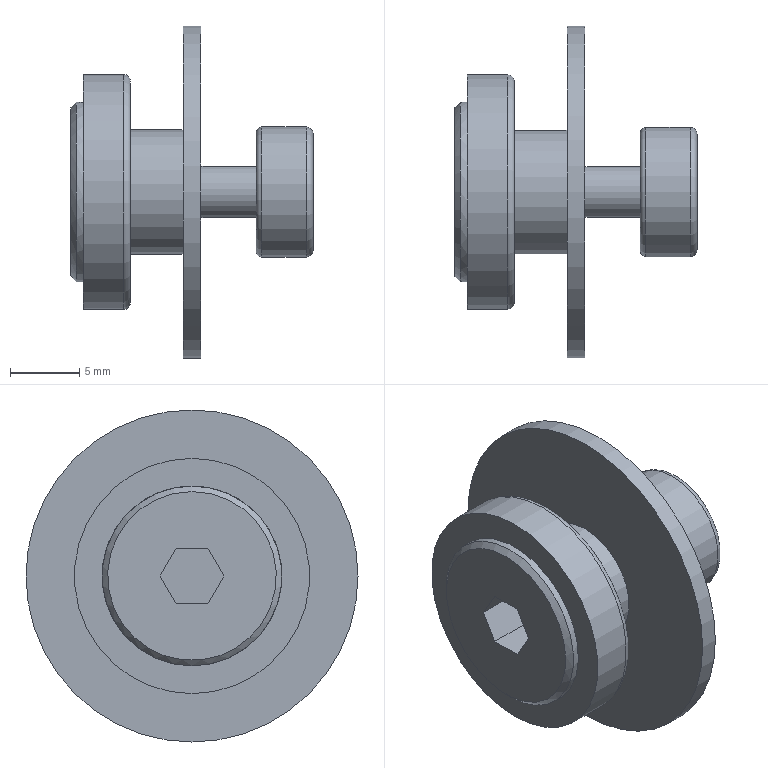Part | STEP file | DEWALT-DWE7492-B22 | 1 solid | 24 faces | box 17.5 x 24 x 24 mm | volume 1970 mm3 | plane 14 | cylinder 6 | torus 3 | cone 1 | commonest cylinder face diameters 3.688 x1 9 x1 9.4 x1 13 x1 17 x1 24 x1